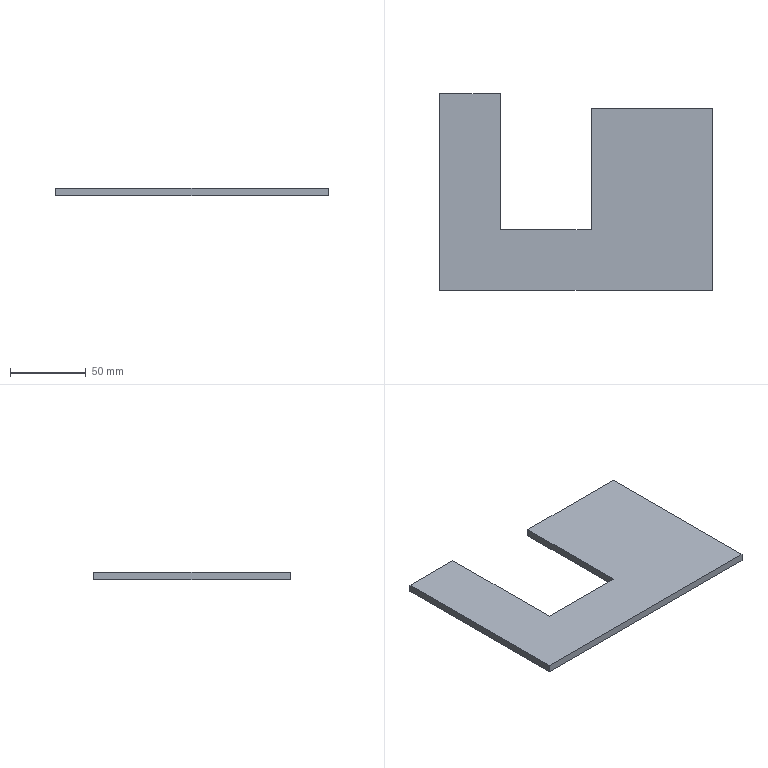Part | SolidWorks | features Extrusion 1 | 1 solid | 10 faces | box 180 x 130 x 5 mm | volume 86000 mm3 | plane 10
STEP:
#1=CARTESIAN_POINT('',(0.,0.,0.));
#2=VERTEX_POINT('',#1);
#3=CARTESIAN_POINT('',(180.,0.,0.));
#4=VERTEX_POINT('',#3);
#5=CARTESIAN_POINT('',(0.,0.,0.));
#6=DIRECTION('',(1.,0.,0.));
#7=VECTOR('',#6,1000.);
#8=LINE('',#5,#7);
#9=EDGE_CURVE('',#2,#4,#8,.T.);
#10=ORIENTED_EDGE('',*,*,#9,.T.);
#11=CARTESIAN_POINT('',(180.,0.,5.));
#12=VERTEX_POINT('',#11);
#13=CARTESIAN_POINT('',(180.,0.,5.));
#14=DIRECTION('',(0.,0.,-1.));
#15=VECTOR('',#14,1000.);
#16=LINE('',#13,#15);
#17=EDGE_CURVE('',#12,#4,#16,.T.);
#18=ORIENTED_EDGE('',*,*,#17,.F.);
#19=CARTESIAN_POINT('',(0.,0.,5.));
#20=VERTEX_POINT('',#19);
#21=CARTESIAN_POINT('',(0.,0.,5.));
#22=DIRECTION('',(1.,0.,0.));
#23=VECTOR('',#22,1000.);
#24=LINE('',#21,#23);
#25=EDGE_CURVE('',#20,#12,#24,.T.);
#26=ORIENTED_EDGE('',*,*,#25,.F.);
#27=CARTESIAN_POINT('',(0.,0.,5.));
#28=DIRECTION('',(0.,0.,-1.));
#29=VECTOR('',#28,1000.);
#30=LINE('',#27,#29);
#31=EDGE_CURVE('',#20,#2,#30,.T.);
#32=ORIENTED_EDGE('',*,*,#31,.T.);
#33=EDGE_LOOP('',(#10,#18,#26,#32));
#34=FACE_OUTER_BOUND('',#33,.T.);
#35=CARTESIAN_POINT('',(0.,0.,5.));
#36=DIRECTION('',(0.,1.,0.));
#37=DIRECTION('',(0.,0.,1.));
#38=AXIS2_PLACEMENT_3D('',#35,#36,#37);
#39=PLANE('',#38);
#40=ADVANCED_FACE('',(#34),#39,.F.);
#41=CARTESIAN_POINT('',(180.,120.,0.));
#42=VERTEX_POINT('',#41);
#43=CARTESIAN_POINT('',(180.,0.,0.));
#44=DIRECTION('',(0.,1.,0.));
#45=VECTOR('',#44,1000.);
#46=LINE('',#43,#45);
#47=EDGE_CURVE('',#4,#42,#46,.T.);
#48=ORIENTED_EDGE('',*,*,#47,.T.);
#49=CARTESIAN_POINT('',(180.,120.,5.));
#50=VERTEX_POINT('',#49);
#51=CARTESIAN_POINT('',(180.,120.,5.));
#52=DIRECTION('',(0.,0.,-1.));
#53=VECTOR('',#52,1000.);
#54=LINE('',#51,#53);
#55=EDGE_CURVE('',#50,#42,#54,.T.);
#56=ORIENTED_EDGE('',*,*,#55,.F.);
#57=CARTESIAN_POINT('',(180.,0.,5.));
#58=DIRECTION('',(0.,1.,0.));
#59=VECTOR('',#58,1000.);
#60=LINE('',#57,#59);
#61=EDGE_CURVE('',#12,#50,#60,.T.);
#62=ORIENTED_EDGE('',*,*,#61,.F.);
#63=ORIENTED_EDGE('',*,*,#17,.T.);
#64=EDGE_LOOP('',(#48,#56,#62,#63));
#65=FACE_OUTER_BOUND('',#64,.T.);
#66=CARTESIAN_POINT('',(180.,0.,5.));
#67=DIRECTION('',(-1.,0.,0.));
#68=DIRECTION('',(0.,0.,1.));
#69=AXIS2_PLACEMENT_3D('',#66,#67,#68);
#70=PLANE('',#69);
#71=ADVANCED_FACE('',(#65),#70,.F.);
#72=CARTESIAN_POINT('',(100.,120.,0.));
#73=VERTEX_POINT('',#72);
#74=CARTESIAN_POINT('',(180.,120.,0.));
#75=DIRECTION('',(-1.,0.,0.));
#76=VECTOR('',#75,1000.);
#77=LINE('',#74,#76);
#78=EDGE_CURVE('',#42,#73,#77,.T.);
#79=ORIENTED_EDGE('',*,*,#78,.T.);
#80=CARTESIAN_POINT('',(100.,120.,5.));
#81=VERTEX_POINT('',#80);
#82=CARTESIAN_POINT('',(100.,120.,5.));
#83=DIRECTION('',(0.,0.,-1.));
#84=VECTOR('',#83,1000.);
#85=LINE('',#82,#84);
#86=EDGE_CURVE('',#81,#73,#85,.T.);
#87=ORIENTED_EDGE('',*,*,#86,.F.);
#88=CARTESIAN_POINT('',(180.,120.,5.));
#89=DIRECTION('',(-1.,0.,0.));
#90=VECTOR('',#89,1000.);
#91=LINE('',#88,#90);
#92=EDGE_CURVE('',#50,#81,#91,.T.);
#93=ORIENTED_EDGE('',*,*,#92,.F.);
#94=ORIENTED_EDGE('',*,*,#55,.T.);
#95=EDGE_LOOP('',(#79,#87,#93,#94));
#96=FACE_OUTER_BOUND('',#95,.T.);
#97=CARTESIAN_POINT('',(180.,120.,5.));
#98=DIRECTION('',(0.,-1.,0.));
#99=DIRECTION('',(1.,0.,0.));
#100=AXIS2_PLACEMENT_3D('',#97,#98,#99);
#101=PLANE('',#100);
#102=ADVANCED_FACE('',(#96),#101,.F.);
#103=CARTESIAN_POINT('',(100.,40.,0.));
#104=VERTEX_POINT('',#103);
#105=CARTESIAN_POINT('',(100.,40.,0.));
#106=DIRECTION('',(0.,-1.,0.));
#107=VECTOR('',#106,1000.);
#108=LINE('',#105,#107);
#109=EDGE_CURVE('',#73,#104,#108,.T.);
#110=ORIENTED_EDGE('',*,*,#109,.T.);
#111=CARTESIAN_POINT('',(100.,40.,5.));
#112=VERTEX_POINT('',#111);
#113=CARTESIAN_POINT('',(100.,40.,5.));
#114=DIRECTION('',(0.,0.,-1.));
#115=VECTOR('',#114,1000.);
#116=LINE('',#113,#115);
#117=EDGE_CURVE('',#112,#104,#116,.T.);
#118=ORIENTED_EDGE('',*,*,#117,.F.);
#119=CARTESIAN_POINT('',(100.,40.,5.));
#120=DIRECTION('',(0.,-1.,0.));
#121=VECTOR('',#120,1000.);
#122=LINE('',#119,#121);
#123=EDGE_CURVE('',#81,#112,#122,.T.);
#124=ORIENTED_EDGE('',*,*,#123,.F.);
#125=ORIENTED_EDGE('',*,*,#86,.T.);
#126=EDGE_LOOP('',(#110,#118,#124,#125));
#127=FACE_OUTER_BOUND('',#126,.T.);
#128=CARTESIAN_POINT('',(100.,40.,5.));
#129=DIRECTION('',(1.,0.,0.));
#130=DIRECTION('',(0.,0.,-1.));
#131=AXIS2_PLACEMENT_3D('',#128,#129,#130);
#132=PLANE('',#131);
#133=ADVANCED_FACE('',(#127),#132,.F.);
#134=CARTESIAN_POINT('',(40.,40.,0.));
#135=VERTEX_POINT('',#134);
#136=CARTESIAN_POINT('',(100.,40.,0.));
#137=DIRECTION('',(-1.,0.,0.));
#138=VECTOR('',#137,1000.);
#139=LINE('',#136,#138);
#140=EDGE_CURVE('',#104,#135,#139,.T.);
#141=ORIENTED_EDGE('',*,*,#140,.T.);
#142=CARTESIAN_POINT('',(40.,40.,5.));
#143=VERTEX_POINT('',#142);
#144=CARTESIAN_POINT('',(40.,40.,5.));
#145=DIRECTION('',(0.,0.,-1.));
#146=VECTOR('',#145,1000.);
#147=LINE('',#144,#146);
#148=EDGE_CURVE('',#143,#135,#147,.T.);
#149=ORIENTED_EDGE('',*,*,#148,.F.);
#150=CARTESIAN_POINT('',(100.,40.,5.));
#151=DIRECTION('',(-1.,0.,0.));
#152=VECTOR('',#151,1000.);
#153=LINE('',#150,#152);
#154=EDGE_CURVE('',#112,#143,#153,.T.);
#155=ORIENTED_EDGE('',*,*,#154,.F.);
#156=ORIENTED_EDGE('',*,*,#117,.T.);
#157=EDGE_LOOP('',(#141,#149,#155,#156));
#158=FACE_OUTER_BOUND('',#157,.T.);
#159=CARTESIAN_POINT('',(100.,40.,5.));
#160=DIRECTION('',(0.,-1.,0.));
#161=DIRECTION('',(0.,0.,-1.));
#162=AXIS2_PLACEMENT_3D('',#159,#160,#161);
#163=PLANE('',#162);
#164=ADVANCED_FACE('',(#158),#163,.F.);
#165=CARTESIAN_POINT('',(40.,130.,0.));
#166=VERTEX_POINT('',#165);
#167=CARTESIAN_POINT('',(40.,130.,0.));
#168=DIRECTION('',(0.,1.,0.));
#169=VECTOR('',#168,1000.);
#170=LINE('',#167,#169);
#171=EDGE_CURVE('',#135,#166,#170,.T.);
#172=ORIENTED_EDGE('',*,*,#171,.T.);
#173=CARTESIAN_POINT('',(40.,130.,5.));
#174=VERTEX_POINT('',#173);
#175=CARTESIAN_POINT('',(40.,130.,5.));
#176=DIRECTION('',(0.,0.,-1.));
#177=VECTOR('',#176,1000.);
#178=LINE('',#175,#177);
#179=EDGE_CURVE('',#174,#166,#178,.T.);
#180=ORIENTED_EDGE('',*,*,#179,.F.);
#181=CARTESIAN_POINT('',(40.,130.,5.));
#182=DIRECTION('',(0.,1.,0.));
#183=VECTOR('',#182,1000.);
#184=LINE('',#181,#183);
#185=EDGE_CURVE('',#143,#174,#184,.T.);
#186=ORIENTED_EDGE('',*,*,#185,.F.);
#187=ORIENTED_EDGE('',*,*,#148,.T.);
#188=EDGE_LOOP('',(#172,#180,#186,#187));
#189=FACE_OUTER_BOUND('',#188,.T.);
#190=CARTESIAN_POINT('',(40.,130.,5.));
#191=DIRECTION('',(-1.,0.,0.));
#192=DIRECTION('',(0.,-1.,0.));
#193=AXIS2_PLACEMENT_3D('',#190,#191,#192);
#194=PLANE('',#193);
#195=ADVANCED_FACE('',(#189),#194,.F.);
#196=CARTESIAN_POINT('',(0.,130.,0.));
#197=VERTEX_POINT('',#196);
#198=CARTESIAN_POINT('',(0.,130.,0.));
#199=DIRECTION('',(-1.,0.,0.));
#200=VECTOR('',#199,1000.);
#201=LINE('',#198,#200);
#202=EDGE_CURVE('',#166,#197,#201,.T.);
#203=ORIENTED_EDGE('',*,*,#202,.T.);
#204=CARTESIAN_POINT('',(0.,130.,5.));
#205=VERTEX_POINT('',#204);
#206=CARTESIAN_POINT('',(0.,130.,5.));
#207=DIRECTION('',(0.,0.,-1.));
#208=VECTOR('',#207,1000.);
#209=LINE('',#206,#208);
#210=EDGE_CURVE('',#205,#197,#209,.T.);
#211=ORIENTED_EDGE('',*,*,#210,.F.);
#212=CARTESIAN_POINT('',(0.,130.,5.));
#213=DIRECTION('',(-1.,0.,0.));
#214=VECTOR('',#213,1000.);
#215=LINE('',#212,#214);
#216=EDGE_CURVE('',#174,#205,#215,.T.);
#217=ORIENTED_EDGE('',*,*,#216,.F.);
#218=ORIENTED_EDGE('',*,*,#179,.T.);
#219=EDGE_LOOP('',(#203,#211,#217,#218));
#220=FACE_OUTER_BOUND('',#219,.T.);
#221=CARTESIAN_POINT('',(0.,130.,5.));
#222=DIRECTION('',(0.,-1.,0.));
#223=DIRECTION('',(0.,0.,-1.));
#224=AXIS2_PLACEMENT_3D('',#221,#222,#223);
#225=PLANE('',#224);
#226=ADVANCED_FACE('',(#220),#225,.F.);
#227=CARTESIAN_POINT('',(0.,0.,0.));
#228=DIRECTION('',(0.,-1.,0.));
#229=VECTOR('',#228,1000.);
#230=LINE('',#227,#229);
#231=EDGE_CURVE('',#197,#2,#230,.T.);
#232=ORIENTED_EDGE('',*,*,#231,.T.);
#233=ORIENTED_EDGE('',*,*,#31,.F.);
#234=CARTESIAN_POINT('',(0.,0.,5.));
#235=DIRECTION('',(0.,-1.,0.));
#236=VECTOR('',#235,1000.);
#237=LINE('',#234,#236);
#238=EDGE_CURVE('',#205,#20,#237,.T.);
#239=ORIENTED_EDGE('',*,*,#238,.F.);
#240=ORIENTED_EDGE('',*,*,#210,.T.);
#241=EDGE_LOOP('',(#232,#233,#239,#240));
#242=FACE_OUTER_BOUND('',#241,.T.);
#243=CARTESIAN_POINT('',(0.,0.,5.));
#244=DIRECTION('',(1.,0.,0.));
#245=DIRECTION('',(0.,0.,-1.));
#246=AXIS2_PLACEMENT_3D('',#243,#244,#245);
#247=PLANE('',#246);
#248=ADVANCED_FACE('',(#242),#247,.F.);
#249=ORIENTED_EDGE('',*,*,#25,.T.);
#250=ORIENTED_EDGE('',*,*,#61,.T.);
#251=ORIENTED_EDGE('',*,*,#92,.T.);
#252=ORIENTED_EDGE('',*,*,#123,.T.);
#253=ORIENTED_EDGE('',*,*,#154,.T.);
#254=ORIENTED_EDGE('',*,*,#185,.T.);
#255=ORIENTED_EDGE('',*,*,#216,.T.);
#256=ORIENTED_EDGE('',*,*,#238,.T.);
#257=EDGE_LOOP('',(#249,#250,#251,#252,#253,#254,#255,#256));
#258=FACE_OUTER_BOUND('',#257,.T.);
#259=CARTESIAN_POINT('',(0.,0.,5.));
#260=DIRECTION('',(0.,0.,1.));
#261=DIRECTION('',(1.,0.,0.));
#262=AXIS2_PLACEMENT_3D('',#259,#260,#261);
#263=PLANE('',#262);
#264=ADVANCED_FACE('',(#258),#263,.T.);
#265=ORIENTED_EDGE('',*,*,#9,.F.);
#266=ORIENTED_EDGE('',*,*,#231,.F.);
#267=ORIENTED_EDGE('',*,*,#202,.F.);
#268=ORIENTED_EDGE('',*,*,#171,.F.);
#269=ORIENTED_EDGE('',*,*,#140,.F.);
#270=ORIENTED_EDGE('',*,*,#109,.F.);
#271=ORIENTED_EDGE('',*,*,#78,.F.);
#272=ORIENTED_EDGE('',*,*,#47,.F.);
#273=EDGE_LOOP('',(#265,#266,#267,#268,#269,#270,#271,#272));
#274=FACE_OUTER_BOUND('',#273,.T.);
#275=CARTESIAN_POINT('',(0.,0.,0.));
#276=DIRECTION('',(0.,0.,1.));
#277=DIRECTION('',(1.,0.,0.));
#278=AXIS2_PLACEMENT_3D('',#275,#276,#277);
#279=PLANE('',#278);
#280=ADVANCED_FACE('',(#274),#279,.F.);
#281=CLOSED_SHELL('',(#40,#71,#102,#133,#164,#195,#226,#248,#264,#280));
#282=MANIFOLD_SOLID_BREP('',#281);
#283=CARTESIAN_POINT('',(0.,0.,0.));
#284=DIRECTION('',(0.,0.,1.));
#285=DIRECTION('',(1.,0.,0.));
#286=AXIS2_PLACEMENT_3D('',#283,#284,#285);
#287=(LENGTH_UNIT()NAMED_UNIT(*)SI_UNIT(.MILLI.,.METRE.));
#288=UNCERTAINTY_MEASURE_WITH_UNIT(LENGTH_MEASURE(0.00001),#287,'','');
#289=(NAMED_UNIT(*)PLANE_ANGLE_UNIT()SI_UNIT($,.RADIAN.));
#290=(NAMED_UNIT(*)SI_UNIT($,.STERADIAN.)SOLID_ANGLE_UNIT());
#291=(GEOMETRIC_REPRESENTATION_CONTEXT(3)GLOBAL_UNCERTAINTY_ASSIGNED_CONTEXT((#288))GLOBAL_UNIT_ASSIGNED_CONTEXT((#287,#289,#290))REPRESENTATION_CONTEXT('',''));
#292=ADVANCED_BREP_SHAPE_REPRESENTATION('',(#282,#286),#291);